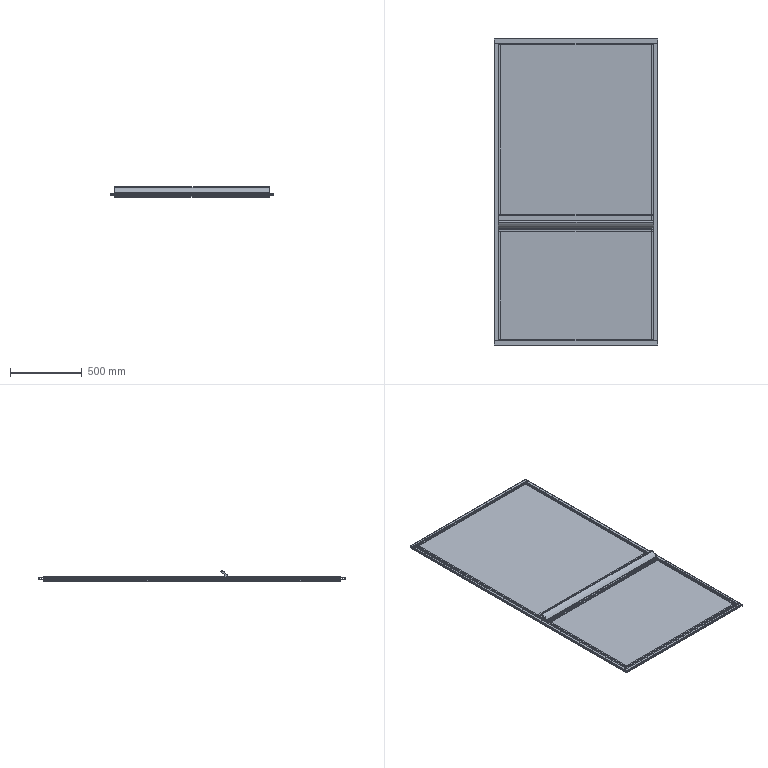Part | SolidWorks | features ICE 13, MirrorSolid 3, LPattern 1, WeldMemberFeat 1, WeldmentFeature 1 | 22 solids | 546 faces | box 1140 x 2136 x 71.386 mm | volume 51691729 mm3 | plane 390 | cylinder 156 | commonest cylinder face diameters 1.1 x36 3.6 x32 5.8 x29 4 x24 1 x10 0.4 x8